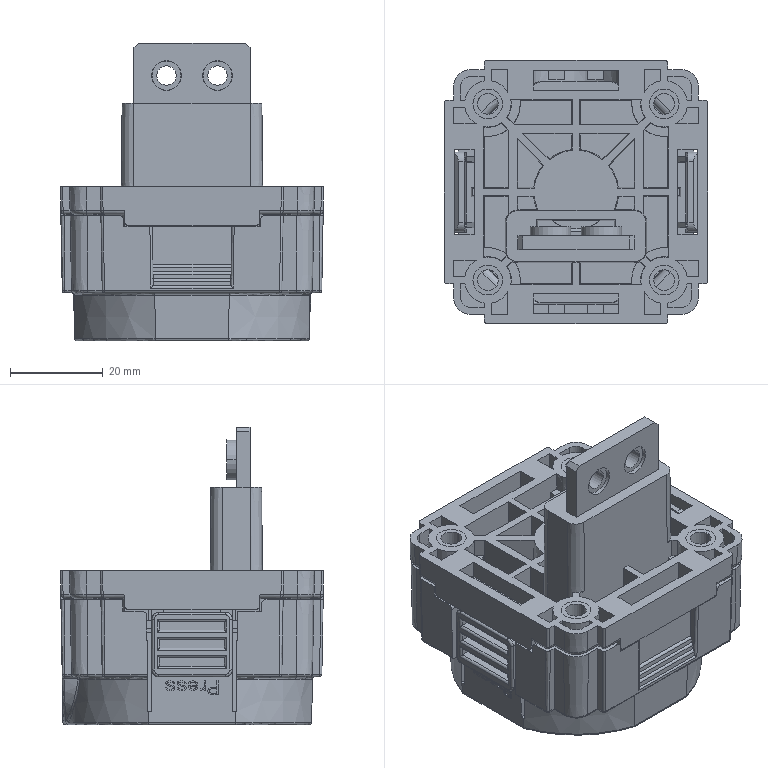Part | NX | features BREP 10 | 10 solids | 2542 faces | box 56.75 x 56.75 x 64.184 mm | volume 46396 mm3 | plane 2185 | cylinder 237 | cone 50 | spline 40 | torus 28 | sphere 2 | commonest cylinder face diameters 1 x75 2 x43 6.4 x20 4 x19 10 x15 3 x8